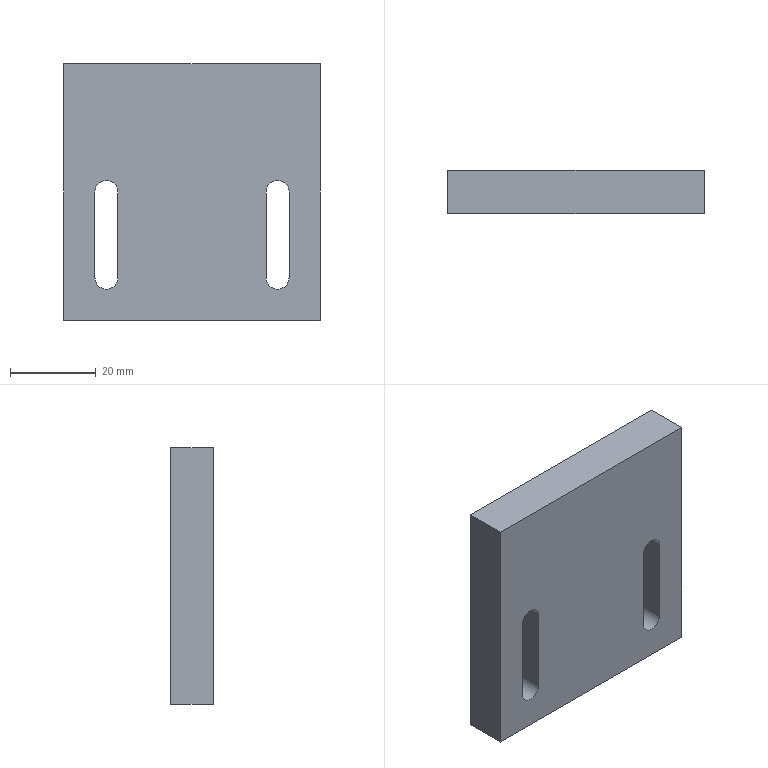Part | SolidWorks | features Cut 1, Extrusion 1, MirrorPattern 1 | 1 solid | 16 faces | box 60 x 10 x 60 mm | volume 33382 mm3 | plane 10 | cylinder 6 | commonest cylinder face diameters 5.4 x6
STEP:
#1=CARTESIAN_POINT('',(-17.3,0.,0.));
#2=VERTEX_POINT('',#1);
#3=CARTESIAN_POINT('',(-20.,0.,2.7));
#4=VERTEX_POINT('',#3);
#5=CARTESIAN_POINT('',(-20.,0.,0.));
#6=DIRECTION('',(0.,-1.,0.));
#7=DIRECTION('',(0.,0.,1.));
#8=AXIS2_PLACEMENT_3D('',#5,#6,#7);
#9=CIRCLE('',#8,2.7);
#10=EDGE_CURVE('',#2,#4,#9,.T.);
#11=ORIENTED_EDGE('',*,*,#10,.T.);
#12=CARTESIAN_POINT('',(-20.,10.,2.7));
#13=VERTEX_POINT('',#12);
#14=CARTESIAN_POINT('',(-20.,0.,2.7));
#15=DIRECTION('',(0.,1.,0.));
#16=VECTOR('',#15,1000.);
#17=LINE('',#14,#16);
#18=EDGE_CURVE('',#4,#13,#17,.T.);
#19=ORIENTED_EDGE('',*,*,#18,.T.);
#20=CARTESIAN_POINT('',(-17.3,10.,0.));
#21=VERTEX_POINT('',#20);
#22=CARTESIAN_POINT('',(-20.,10.,0.));
#23=DIRECTION('',(0.,-1.,0.));
#24=DIRECTION('',(0.,0.,1.));
#25=AXIS2_PLACEMENT_3D('',#22,#23,#24);
#26=CIRCLE('',#25,2.7);
#27=EDGE_CURVE('',#21,#13,#26,.T.);
#28=ORIENTED_EDGE('',*,*,#27,.F.);
#29=CARTESIAN_POINT('',(-17.3,0.,0.));
#30=DIRECTION('',(0.,1.,0.));
#31=VECTOR('',#30,1000.);
#32=LINE('',#29,#31);
#33=EDGE_CURVE('',#2,#21,#32,.T.);
#34=ORIENTED_EDGE('',*,*,#33,.F.);
#35=EDGE_LOOP('',(#11,#19,#28,#34));
#36=FACE_OUTER_BOUND('',#35,.T.);
#37=CARTESIAN_POINT('',(-20.,0.,0.));
#38=DIRECTION('',(0.,1.,0.));
#39=DIRECTION('',(0.,0.,1.));
#40=AXIS2_PLACEMENT_3D('',#37,#38,#39);
#41=CYLINDRICAL_SURFACE('',#40,2.7);
#42=ADVANCED_FACE('',(#36),#41,.F.);
#43=CARTESIAN_POINT('',(20.,0.,2.7));
#44=VERTEX_POINT('',#43);
#45=CARTESIAN_POINT('',(22.7,0.,0.));
#46=VERTEX_POINT('',#45);
#47=CARTESIAN_POINT('',(20.,0.,0.));
#48=DIRECTION('',(0.,1.,0.));
#49=DIRECTION('',(0.,0.,1.));
#50=AXIS2_PLACEMENT_3D('',#47,#48,#49);
#51=CIRCLE('',#50,2.7);
#52=EDGE_CURVE('',#44,#46,#51,.T.);
#53=ORIENTED_EDGE('',*,*,#52,.F.);
#54=CARTESIAN_POINT('',(20.,10.,2.7));
#55=VERTEX_POINT('',#54);
#56=CARTESIAN_POINT('',(20.,0.,2.7));
#57=DIRECTION('',(0.,1.,0.));
#58=VECTOR('',#57,1000.);
#59=LINE('',#56,#58);
#60=EDGE_CURVE('',#44,#55,#59,.T.);
#61=ORIENTED_EDGE('',*,*,#60,.T.);
#62=CARTESIAN_POINT('',(22.7,10.,0.));
#63=VERTEX_POINT('',#62);
#64=CARTESIAN_POINT('',(20.,10.,0.));
#65=DIRECTION('',(0.,1.,0.));
#66=DIRECTION('',(0.,0.,1.));
#67=AXIS2_PLACEMENT_3D('',#64,#65,#66);
#68=CIRCLE('',#67,2.7);
#69=EDGE_CURVE('',#55,#63,#68,.T.);
#70=ORIENTED_EDGE('',*,*,#69,.T.);
#71=CARTESIAN_POINT('',(22.7,0.,0.));
#72=DIRECTION('',(0.,1.,0.));
#73=VECTOR('',#72,1000.);
#74=LINE('',#71,#73);
#75=EDGE_CURVE('',#46,#63,#74,.T.);
#76=ORIENTED_EDGE('',*,*,#75,.F.);
#77=EDGE_LOOP('',(#53,#61,#70,#76));
#78=FACE_OUTER_BOUND('',#77,.T.);
#79=CARTESIAN_POINT('',(20.,0.,0.));
#80=DIRECTION('',(0.,1.,0.));
#81=DIRECTION('',(0.,0.,1.));
#82=AXIS2_PLACEMENT_3D('',#79,#80,#81);
#83=CYLINDRICAL_SURFACE('',#82,2.7);
#84=ADVANCED_FACE('',(#78),#83,.F.);
#85=CARTESIAN_POINT('',(30.,10.,30.));
#86=VERTEX_POINT('',#85);
#87=CARTESIAN_POINT('',(30.,10.,-30.));
#88=VERTEX_POINT('',#87);
#89=CARTESIAN_POINT('',(30.,10.,-30.));
#90=DIRECTION('',(0.,0.,-1.));
#91=VECTOR('',#90,1000.);
#92=LINE('',#89,#91);
#93=EDGE_CURVE('',#86,#88,#92,.T.);
#94=ORIENTED_EDGE('',*,*,#93,.T.);
#95=CARTESIAN_POINT('',(-30.,10.,-30.));
#96=VERTEX_POINT('',#95);
#97=CARTESIAN_POINT('',(-30.,10.,-30.));
#98=DIRECTION('',(-1.,0.,0.));
#99=VECTOR('',#98,1000.);
#100=LINE('',#97,#99);
#101=EDGE_CURVE('',#88,#96,#100,.T.);
#102=ORIENTED_EDGE('',*,*,#101,.T.);
#103=CARTESIAN_POINT('',(-30.,10.,30.));
#104=VERTEX_POINT('',#103);
#105=CARTESIAN_POINT('',(-30.,10.,-30.));
#106=DIRECTION('',(0.,0.,1.));
#107=VECTOR('',#106,1000.);
#108=LINE('',#105,#107);
#109=EDGE_CURVE('',#96,#104,#108,.T.);
#110=ORIENTED_EDGE('',*,*,#109,.T.);
#111=CARTESIAN_POINT('',(-30.,10.,30.));
#112=DIRECTION('',(1.,0.,0.));
#113=VECTOR('',#112,1000.);
#114=LINE('',#111,#113);
#115=EDGE_CURVE('',#104,#86,#114,.T.);
#116=ORIENTED_EDGE('',*,*,#115,.T.);
#117=EDGE_LOOP('',(#94,#102,#110,#116));
#118=FACE_OUTER_BOUND('',#117,.T.);
#119=CARTESIAN_POINT('',(17.3,10.,0.));
#120=VERTEX_POINT('',#119);
#121=CARTESIAN_POINT('',(20.,10.,0.));
#122=DIRECTION('',(0.,1.,0.));
#123=DIRECTION('',(0.,0.,1.));
#124=AXIS2_PLACEMENT_3D('',#121,#122,#123);
#125=CIRCLE('',#124,2.7);
#126=EDGE_CURVE('',#120,#55,#125,.T.);
#127=ORIENTED_EDGE('',*,*,#126,.F.);
#128=CARTESIAN_POINT('',(17.3,10.,-20.));
#129=VERTEX_POINT('',#128);
#130=CARTESIAN_POINT('',(17.3,10.,0.));
#131=DIRECTION('',(0.,0.,1.));
#132=VECTOR('',#131,1000.);
#133=LINE('',#130,#132);
#134=EDGE_CURVE('',#129,#120,#133,.T.);
#135=ORIENTED_EDGE('',*,*,#134,.F.);
#136=CARTESIAN_POINT('',(22.7,10.,-20.));
#137=VERTEX_POINT('',#136);
#138=CARTESIAN_POINT('',(20.,10.,-20.));
#139=DIRECTION('',(0.,1.,0.));
#140=DIRECTION('',(0.,0.,1.));
#141=AXIS2_PLACEMENT_3D('',#138,#139,#140);
#142=CIRCLE('',#141,2.7);
#143=EDGE_CURVE('',#137,#129,#142,.T.);
#144=ORIENTED_EDGE('',*,*,#143,.F.);
#145=CARTESIAN_POINT('',(22.7,10.,0.));
#146=DIRECTION('',(0.,0.,-1.));
#147=VECTOR('',#146,1000.);
#148=LINE('',#145,#147);
#149=EDGE_CURVE('',#63,#137,#148,.T.);
#150=ORIENTED_EDGE('',*,*,#149,.F.);
#151=ORIENTED_EDGE('',*,*,#69,.F.);
#152=EDGE_LOOP('',(#127,#135,#144,#150,#151));
#153=FACE_BOUND('',#152,.T.);
#154=CARTESIAN_POINT('',(-17.3,10.,-20.));
#155=VERTEX_POINT('',#154);
#156=CARTESIAN_POINT('',(-17.3,10.,0.));
#157=DIRECTION('',(0.,0.,1.));
#158=VECTOR('',#157,1000.);
#159=LINE('',#156,#158);
#160=EDGE_CURVE('',#155,#21,#159,.T.);
#161=ORIENTED_EDGE('',*,*,#160,.T.);
#162=ORIENTED_EDGE('',*,*,#27,.T.);
#163=CARTESIAN_POINT('',(-22.7,10.,0.));
#164=VERTEX_POINT('',#163);
#165=CARTESIAN_POINT('',(-20.,10.,0.));
#166=DIRECTION('',(0.,-1.,0.));
#167=DIRECTION('',(0.,0.,1.));
#168=AXIS2_PLACEMENT_3D('',#165,#166,#167);
#169=CIRCLE('',#168,2.7);
#170=EDGE_CURVE('',#13,#164,#169,.T.);
#171=ORIENTED_EDGE('',*,*,#170,.T.);
#172=CARTESIAN_POINT('',(-22.7,10.,-20.));
#173=VERTEX_POINT('',#172);
#174=CARTESIAN_POINT('',(-22.7,10.,0.));
#175=DIRECTION('',(0.,0.,-1.));
#176=VECTOR('',#175,1000.);
#177=LINE('',#174,#176);
#178=EDGE_CURVE('',#164,#173,#177,.T.);
#179=ORIENTED_EDGE('',*,*,#178,.T.);
#180=CARTESIAN_POINT('',(-20.,10.,-20.));
#181=DIRECTION('',(0.,-1.,0.));
#182=DIRECTION('',(0.,0.,1.));
#183=AXIS2_PLACEMENT_3D('',#180,#181,#182);
#184=CIRCLE('',#183,2.7);
#185=EDGE_CURVE('',#173,#155,#184,.T.);
#186=ORIENTED_EDGE('',*,*,#185,.T.);
#187=EDGE_LOOP('',(#161,#162,#171,#179,#186));
#188=FACE_BOUND('',#187,.T.);
#189=CARTESIAN_POINT('',(0.,10.,0.));
#190=DIRECTION('',(0.,1.,0.));
#191=DIRECTION('',(0.,0.,1.));
#192=AXIS2_PLACEMENT_3D('',#189,#190,#191);
#193=PLANE('',#192);
#194=ADVANCED_FACE('',(#118,#153,#188),#193,.T.);
#195=CARTESIAN_POINT('',(30.,0.,30.));
#196=VERTEX_POINT('',#195);
#197=CARTESIAN_POINT('',(30.,0.,-30.));
#198=VERTEX_POINT('',#197);
#199=CARTESIAN_POINT('',(30.,0.,-30.));
#200=DIRECTION('',(0.,0.,-1.));
#201=VECTOR('',#200,1000.);
#202=LINE('',#199,#201);
#203=EDGE_CURVE('',#196,#198,#202,.T.);
#204=ORIENTED_EDGE('',*,*,#203,.F.);
#205=CARTESIAN_POINT('',(-30.,0.,30.));
#206=VERTEX_POINT('',#205);
#207=CARTESIAN_POINT('',(-30.,0.,30.));
#208=DIRECTION('',(1.,0.,0.));
#209=VECTOR('',#208,1000.);
#210=LINE('',#207,#209);
#211=EDGE_CURVE('',#206,#196,#210,.T.);
#212=ORIENTED_EDGE('',*,*,#211,.F.);
#213=CARTESIAN_POINT('',(-30.,0.,-30.));
#214=VERTEX_POINT('',#213);
#215=CARTESIAN_POINT('',(-30.,0.,-30.));
#216=DIRECTION('',(0.,0.,1.));
#217=VECTOR('',#216,1000.);
#218=LINE('',#215,#217);
#219=EDGE_CURVE('',#214,#206,#218,.T.);
#220=ORIENTED_EDGE('',*,*,#219,.F.);
#221=CARTESIAN_POINT('',(-30.,0.,-30.));
#222=DIRECTION('',(-1.,0.,0.));
#223=VECTOR('',#222,1000.);
#224=LINE('',#221,#223);
#225=EDGE_CURVE('',#198,#214,#224,.T.);
#226=ORIENTED_EDGE('',*,*,#225,.F.);
#227=EDGE_LOOP('',(#204,#212,#220,#226));
#228=FACE_OUTER_BOUND('',#227,.T.);
#229=CARTESIAN_POINT('',(17.3,0.,-20.));
#230=VERTEX_POINT('',#229);
#231=CARTESIAN_POINT('',(17.3,0.,0.));
#232=VERTEX_POINT('',#231);
#233=CARTESIAN_POINT('',(17.3,0.,0.));
#234=DIRECTION('',(0.,0.,1.));
#235=VECTOR('',#234,1000.);
#236=LINE('',#233,#235);
#237=EDGE_CURVE('',#230,#232,#236,.T.);
#238=ORIENTED_EDGE('',*,*,#237,.T.);
#239=CARTESIAN_POINT('',(20.,0.,0.));
#240=DIRECTION('',(0.,1.,0.));
#241=DIRECTION('',(0.,0.,1.));
#242=AXIS2_PLACEMENT_3D('',#239,#240,#241);
#243=CIRCLE('',#242,2.7);
#244=EDGE_CURVE('',#232,#44,#243,.T.);
#245=ORIENTED_EDGE('',*,*,#244,.T.);
#246=ORIENTED_EDGE('',*,*,#52,.T.);
#247=CARTESIAN_POINT('',(22.7,0.,-20.));
#248=VERTEX_POINT('',#247);
#249=CARTESIAN_POINT('',(22.7,0.,0.));
#250=DIRECTION('',(0.,0.,-1.));
#251=VECTOR('',#250,1000.);
#252=LINE('',#249,#251);
#253=EDGE_CURVE('',#46,#248,#252,.T.);
#254=ORIENTED_EDGE('',*,*,#253,.T.);
#255=CARTESIAN_POINT('',(20.,0.,-20.));
#256=DIRECTION('',(0.,1.,0.));
#257=DIRECTION('',(0.,0.,1.));
#258=AXIS2_PLACEMENT_3D('',#255,#256,#257);
#259=CIRCLE('',#258,2.7);
#260=EDGE_CURVE('',#248,#230,#259,.T.);
#261=ORIENTED_EDGE('',*,*,#260,.T.);
#262=EDGE_LOOP('',(#238,#245,#246,#254,#261));
#263=FACE_BOUND('',#262,.T.);
#264=ORIENTED_EDGE('',*,*,#10,.F.);
#265=CARTESIAN_POINT('',(-17.3,0.,-20.));
#266=VERTEX_POINT('',#265);
#267=CARTESIAN_POINT('',(-17.3,0.,0.));
#268=DIRECTION('',(0.,0.,1.));
#269=VECTOR('',#268,1000.);
#270=LINE('',#267,#269);
#271=EDGE_CURVE('',#266,#2,#270,.T.);
#272=ORIENTED_EDGE('',*,*,#271,.F.);
#273=CARTESIAN_POINT('',(-22.7,0.,-20.));
#274=VERTEX_POINT('',#273);
#275=CARTESIAN_POINT('',(-20.,0.,-20.));
#276=DIRECTION('',(0.,-1.,0.));
#277=DIRECTION('',(0.,0.,1.));
#278=AXIS2_PLACEMENT_3D('',#275,#276,#277);
#279=CIRCLE('',#278,2.7);
#280=EDGE_CURVE('',#274,#266,#279,.T.);
#281=ORIENTED_EDGE('',*,*,#280,.F.);
#282=CARTESIAN_POINT('',(-22.7,0.,0.));
#283=VERTEX_POINT('',#282);
#284=CARTESIAN_POINT('',(-22.7,0.,0.));
#285=DIRECTION('',(0.,0.,-1.));
#286=VECTOR('',#285,1000.);
#287=LINE('',#284,#286);
#288=EDGE_CURVE('',#283,#274,#287,.T.);
#289=ORIENTED_EDGE('',*,*,#288,.F.);
#290=CARTESIAN_POINT('',(-20.,0.,0.));
#291=DIRECTION('',(0.,-1.,0.));
#292=DIRECTION('',(0.,0.,1.));
#293=AXIS2_PLACEMENT_3D('',#290,#291,#292);
#294=CIRCLE('',#293,2.7);
#295=EDGE_CURVE('',#4,#283,#294,.T.);
#296=ORIENTED_EDGE('',*,*,#295,.F.);
#297=EDGE_LOOP('',(#264,#272,#281,#289,#296));
#298=FACE_BOUND('',#297,.T.);
#299=CARTESIAN_POINT('',(0.,0.,0.));
#300=DIRECTION('',(0.,1.,0.));
#301=DIRECTION('',(0.,0.,1.));
#302=AXIS2_PLACEMENT_3D('',#299,#300,#301);
#303=PLANE('',#302);
#304=ADVANCED_FACE('',(#228,#263,#298),#303,.F.);
#305=ORIENTED_EDGE('',*,*,#203,.T.);
#306=CARTESIAN_POINT('',(30.,10.,-30.));
#307=DIRECTION('',(0.,-1.,0.));
#308=VECTOR('',#307,1000.);
#309=LINE('',#306,#308);
#310=EDGE_CURVE('',#88,#198,#309,.T.);
#311=ORIENTED_EDGE('',*,*,#310,.F.);
#312=ORIENTED_EDGE('',*,*,#93,.F.);
#313=CARTESIAN_POINT('',(30.,10.,30.));
#314=DIRECTION('',(0.,-1.,0.));
#315=VECTOR('',#314,1000.);
#316=LINE('',#313,#315);
#317=EDGE_CURVE('',#86,#196,#316,.T.);
#318=ORIENTED_EDGE('',*,*,#317,.T.);
#319=EDGE_LOOP('',(#305,#311,#312,#318));
#320=FACE_OUTER_BOUND('',#319,.T.);
#321=CARTESIAN_POINT('',(30.,10.,-30.));
#322=DIRECTION('',(-1.,0.,0.));
#323=DIRECTION('',(0.,0.,1.));
#324=AXIS2_PLACEMENT_3D('',#321,#322,#323);
#325=PLANE('',#324);
#326=ADVANCED_FACE('',(#320),#325,.F.);
#327=ORIENTED_EDGE('',*,*,#225,.T.);
#328=CARTESIAN_POINT('',(-30.,10.,-30.));
#329=DIRECTION('',(0.,-1.,0.));
#330=VECTOR('',#329,1000.);
#331=LINE('',#328,#330);
#332=EDGE_CURVE('',#96,#214,#331,.T.);
#333=ORIENTED_EDGE('',*,*,#332,.F.);
#334=ORIENTED_EDGE('',*,*,#101,.F.);
#335=ORIENTED_EDGE('',*,*,#310,.T.);
#336=EDGE_LOOP('',(#327,#333,#334,#335));
#337=FACE_OUTER_BOUND('',#336,.T.);
#338=CARTESIAN_POINT('',(-30.,10.,-30.));
#339=DIRECTION('',(0.,0.,1.));
#340=DIRECTION('',(1.,0.,0.));
#341=AXIS2_PLACEMENT_3D('',#338,#339,#340);
#342=PLANE('',#341);
#343=ADVANCED_FACE('',(#337),#342,.F.);
#344=ORIENTED_EDGE('',*,*,#219,.T.);
#345=CARTESIAN_POINT('',(-30.,10.,30.));
#346=DIRECTION('',(0.,-1.,0.));
#347=VECTOR('',#346,1000.);
#348=LINE('',#345,#347);
#349=EDGE_CURVE('',#104,#206,#348,.T.);
#350=ORIENTED_EDGE('',*,*,#349,.F.);
#351=ORIENTED_EDGE('',*,*,#109,.F.);
#352=ORIENTED_EDGE('',*,*,#332,.T.);
#353=EDGE_LOOP('',(#344,#350,#351,#352));
#354=FACE_OUTER_BOUND('',#353,.T.);
#355=CARTESIAN_POINT('',(-30.,10.,-30.));
#356=DIRECTION('',(1.,0.,0.));
#357=DIRECTION('',(0.,0.,-1.));
#358=AXIS2_PLACEMENT_3D('',#355,#356,#357);
#359=PLANE('',#358);
#360=ADVANCED_FACE('',(#354),#359,.F.);
#361=ORIENTED_EDGE('',*,*,#211,.T.);
#362=ORIENTED_EDGE('',*,*,#317,.F.);
#363=ORIENTED_EDGE('',*,*,#115,.F.);
#364=ORIENTED_EDGE('',*,*,#349,.T.);
#365=EDGE_LOOP('',(#361,#362,#363,#364));
#366=FACE_OUTER_BOUND('',#365,.T.);
#367=CARTESIAN_POINT('',(-30.,10.,30.));
#368=DIRECTION('',(0.,0.,-1.));
#369=DIRECTION('',(-1.,0.,0.));
#370=AXIS2_PLACEMENT_3D('',#367,#368,#369);
#371=PLANE('',#370);
#372=ADVANCED_FACE('',(#366),#371,.F.);
#373=ORIENTED_EDGE('',*,*,#60,.F.);
#374=ORIENTED_EDGE('',*,*,#244,.F.);
#375=CARTESIAN_POINT('',(17.3,0.,0.));
#376=DIRECTION('',(0.,1.,0.));
#377=VECTOR('',#376,1000.);
#378=LINE('',#375,#377);
#379=EDGE_CURVE('',#232,#120,#378,.T.);
#380=ORIENTED_EDGE('',*,*,#379,.T.);
#381=ORIENTED_EDGE('',*,*,#126,.T.);
#382=EDGE_LOOP('',(#373,#374,#380,#381));
#383=FACE_OUTER_BOUND('',#382,.T.);
#384=CARTESIAN_POINT('',(20.,0.,0.));
#385=DIRECTION('',(0.,1.,0.));
#386=DIRECTION('',(0.,0.,1.));
#387=AXIS2_PLACEMENT_3D('',#384,#385,#386);
#388=CYLINDRICAL_SURFACE('',#387,2.7);
#389=ADVANCED_FACE('',(#383),#388,.F.);
#390=ORIENTED_EDGE('',*,*,#134,.T.);
#391=ORIENTED_EDGE('',*,*,#379,.F.);
#392=ORIENTED_EDGE('',*,*,#237,.F.);
#393=CARTESIAN_POINT('',(17.3,0.,-20.));
#394=DIRECTION('',(0.,1.,0.));
#395=VECTOR('',#394,1000.);
#396=LINE('',#393,#395);
#397=EDGE_CURVE('',#230,#129,#396,.T.);
#398=ORIENTED_EDGE('',*,*,#397,.T.);
#399=EDGE_LOOP('',(#390,#391,#392,#398));
#400=FACE_OUTER_BOUND('',#399,.T.);
#401=CARTESIAN_POINT('',(17.3,0.,0.));
#402=DIRECTION('',(-1.,0.,0.));
#403=DIRECTION('',(0.,0.,1.));
#404=AXIS2_PLACEMENT_3D('',#401,#402,#403);
#405=PLANE('',#404);
#406=ADVANCED_FACE('',(#400),#405,.F.);
#407=ORIENTED_EDGE('',*,*,#143,.T.);
#408=ORIENTED_EDGE('',*,*,#397,.F.);
#409=ORIENTED_EDGE('',*,*,#260,.F.);
#410=CARTESIAN_POINT('',(22.7,0.,-20.));
#411=DIRECTION('',(0.,1.,0.));
#412=VECTOR('',#411,1000.);
#413=LINE('',#410,#412);
#414=EDGE_CURVE('',#248,#137,#413,.T.);
#415=ORIENTED_EDGE('',*,*,#414,.T.);
#416=EDGE_LOOP('',(#407,#408,#409,#415));
#417=FACE_OUTER_BOUND('',#416,.T.);
#418=CARTESIAN_POINT('',(20.,0.,-20.));
#419=DIRECTION('',(0.,1.,0.));
#420=DIRECTION('',(0.,0.,1.));
#421=AXIS2_PLACEMENT_3D('',#418,#419,#420);
#422=CYLINDRICAL_SURFACE('',#421,2.7);
#423=ADVANCED_FACE('',(#417),#422,.F.);
#424=ORIENTED_EDGE('',*,*,#149,.T.);
#425=ORIENTED_EDGE('',*,*,#414,.F.);
#426=ORIENTED_EDGE('',*,*,#253,.F.);
#427=ORIENTED_EDGE('',*,*,#75,.T.);
#428=EDGE_LOOP('',(#424,#425,#426,#427));
#429=FACE_OUTER_BOUND('',#428,.T.);
#430=CARTESIAN_POINT('',(22.7,0.,0.));
#431=DIRECTION('',(1.,0.,0.));
#432=DIRECTION('',(0.,0.,-1.));
#433=AXIS2_PLACEMENT_3D('',#430,#431,#432);
#434=PLANE('',#433);
#435=ADVANCED_FACE('',(#429),#434,.F.);
#436=ORIENTED_EDGE('',*,*,#18,.F.);
#437=ORIENTED_EDGE('',*,*,#295,.T.);
#438=CARTESIAN_POINT('',(-22.7,0.,0.));
#439=DIRECTION('',(0.,1.,0.));
#440=VECTOR('',#439,1000.);
#441=LINE('',#438,#440);
#442=EDGE_CURVE('',#283,#164,#441,.T.);
#443=ORIENTED_EDGE('',*,*,#442,.T.);
#444=ORIENTED_EDGE('',*,*,#170,.F.);
#445=EDGE_LOOP('',(#436,#437,#443,#444));
#446=FACE_OUTER_BOUND('',#445,.T.);
#447=CARTESIAN_POINT('',(-20.,0.,0.));
#448=DIRECTION('',(0.,1.,0.));
#449=DIRECTION('',(0.,0.,1.));
#450=AXIS2_PLACEMENT_3D('',#447,#448,#449);
#451=CYLINDRICAL_SURFACE('',#450,2.7);
#452=ADVANCED_FACE('',(#446),#451,.F.);
#453=ORIENTED_EDGE('',*,*,#178,.F.);
#454=ORIENTED_EDGE('',*,*,#442,.F.);
#455=ORIENTED_EDGE('',*,*,#288,.T.);
#456=CARTESIAN_POINT('',(-22.7,0.,-20.));
#457=DIRECTION('',(0.,1.,0.));
#458=VECTOR('',#457,1000.);
#459=LINE('',#456,#458);
#460=EDGE_CURVE('',#274,#173,#459,.T.);
#461=ORIENTED_EDGE('',*,*,#460,.T.);
#462=EDGE_LOOP('',(#453,#454,#455,#461));
#463=FACE_OUTER_BOUND('',#462,.T.);
#464=CARTESIAN_POINT('',(-22.7,0.,0.));
#465=DIRECTION('',(1.,0.,0.));
#466=DIRECTION('',(0.,0.,-1.));
#467=AXIS2_PLACEMENT_3D('',#464,#465,#466);
#468=PLANE('',#467);
#469=ADVANCED_FACE('',(#463),#468,.T.);
#470=ORIENTED_EDGE('',*,*,#185,.F.);
#471=ORIENTED_EDGE('',*,*,#460,.F.);
#472=ORIENTED_EDGE('',*,*,#280,.T.);
#473=CARTESIAN_POINT('',(-17.3,0.,-20.));
#474=DIRECTION('',(0.,1.,0.));
#475=VECTOR('',#474,1000.);
#476=LINE('',#473,#475);
#477=EDGE_CURVE('',#266,#155,#476,.T.);
#478=ORIENTED_EDGE('',*,*,#477,.T.);
#479=EDGE_LOOP('',(#470,#471,#472,#478));
#480=FACE_OUTER_BOUND('',#479,.T.);
#481=CARTESIAN_POINT('',(-20.,0.,-20.));
#482=DIRECTION('',(0.,1.,0.));
#483=DIRECTION('',(0.,0.,1.));
#484=AXIS2_PLACEMENT_3D('',#481,#482,#483);
#485=CYLINDRICAL_SURFACE('',#484,2.7);
#486=ADVANCED_FACE('',(#480),#485,.F.);
#487=ORIENTED_EDGE('',*,*,#160,.F.);
#488=ORIENTED_EDGE('',*,*,#477,.F.);
#489=ORIENTED_EDGE('',*,*,#271,.T.);
#490=ORIENTED_EDGE('',*,*,#33,.T.);
#491=EDGE_LOOP('',(#487,#488,#489,#490));
#492=FACE_OUTER_BOUND('',#491,.T.);
#493=CARTESIAN_POINT('',(-17.3,0.,0.));
#494=DIRECTION('',(-1.,0.,0.));
#495=DIRECTION('',(0.,0.,1.));
#496=AXIS2_PLACEMENT_3D('',#493,#494,#495);
#497=PLANE('',#496);
#498=ADVANCED_FACE('',(#492),#497,.T.);
#499=CLOSED_SHELL('',(#42,#84,#194,#304,#326,#343,#360,#372,#389,#406,#423,#435,#452,#469,#486,#498));
#500=MANIFOLD_SOLID_BREP('',#499);
#501=CARTESIAN_POINT('',(0.,0.,0.));
#502=DIRECTION('',(0.,0.,1.));
#503=DIRECTION('',(1.,0.,0.));
#504=AXIS2_PLACEMENT_3D('',#501,#502,#503);
#505=(LENGTH_UNIT()NAMED_UNIT(*)SI_UNIT(.MILLI.,.METRE.));
#506=UNCERTAINTY_MEASURE_WITH_UNIT(LENGTH_MEASURE(0.00001),#505,'','');
#507=(NAMED_UNIT(*)PLANE_ANGLE_UNIT()SI_UNIT($,.RADIAN.));
#508=(NAMED_UNIT(*)SI_UNIT($,.STERADIAN.)SOLID_ANGLE_UNIT());
#509=(GEOMETRIC_REPRESENTATION_CONTEXT(3)GLOBAL_UNCERTAINTY_ASSIGNED_CONTEXT((#506))GLOBAL_UNIT_ASSIGNED_CONTEXT((#505,#507,#508))REPRESENTATION_CONTEXT('',''));
#510=ADVANCED_BREP_SHAPE_REPRESENTATION('',(#500,#504),#509);